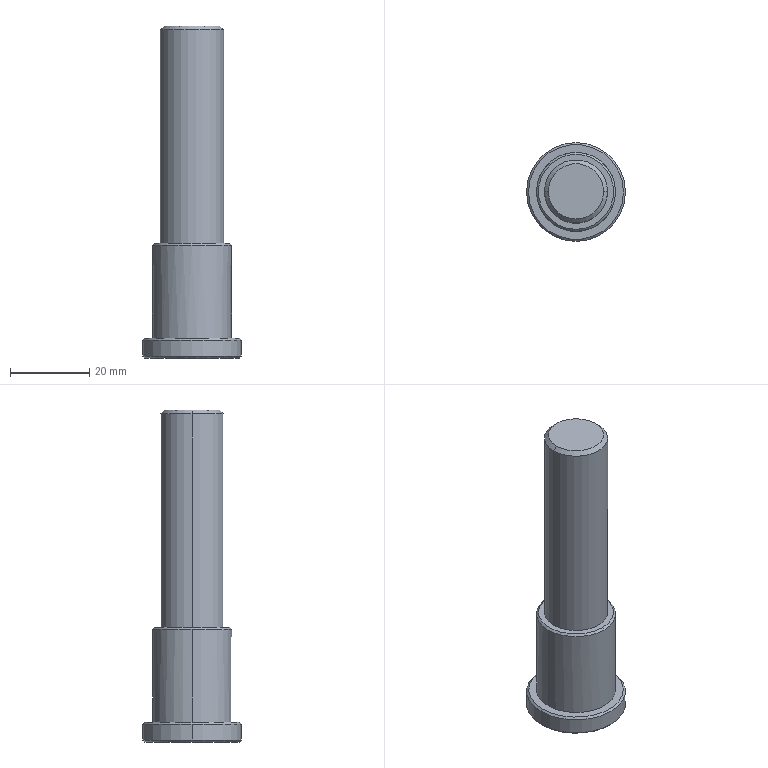Part | STEP file | 1 solid | 18 faces | box 25 x 25 x 84 mm | volume 21001 mm3 | cone 8 | cylinder 6 | plane 4 | commonest cylinder face diameters 16 x2 20 x2 25 x2
STEP:
#1=CARTESIAN_POINT('',(0.,0.,0.));
#2=DIRECTION('',(0.,0.,1.));
#3=DIRECTION('',(1.,0.,0.));
#4=AXIS2_PLACEMENT_3D('',#1,#2,#3);
#5=CARTESIAN_POINT('',(12.,0.,0.));
#6=VERTEX_POINT('',#5);
#7=CARTESIAN_POINT('',(-12.,0.,0.));
#8=VERTEX_POINT('',#7);
#9=CARTESIAN_POINT('',(0.,0.,0.));
#10=DIRECTION('',(0.,0.,1.));
#11=DIRECTION('',(1.,0.,0.));
#12=AXIS2_PLACEMENT_3D('',#9,#10,#11);
#13=CIRCLE('',#12,12.);
#14=CARTESIAN_POINT('',(0.,0.,0.));
#15=DIRECTION('',(0.,0.,1.));
#16=DIRECTION('',(1.,0.,0.));
#17=AXIS2_PLACEMENT_3D('',#14,#15,#16);
#18=PLANE('',#17);
#19=CARTESIAN_POINT('',(0.,0.));
#20=DIRECTION('',(1.,0.));
#21=AXIS2_PLACEMENT_2D('',#19,#20);
#22=CIRCLE('',#21,12.);
#23=(GEOMETRIC_REPRESENTATION_CONTEXT(2)PARAMETRIC_REPRESENTATION_CONTEXT()REPRESENTATION_CONTEXT('',''));
#24=DEFINITIONAL_REPRESENTATION('',(#22),#23);
#25=PCURVE('',#18,#24);
#26=CARTESIAN_POINT('',(0.,0.,0.5));
#27=DIRECTION('',(0.,0.,1.));
#28=DIRECTION('',(1.,0.,0.));
#29=AXIS2_PLACEMENT_3D('',#26,#27,#28);
#30=CONICAL_SURFACE('',#29,12.5,0.7854);
#31=CARTESIAN_POINT('',(0.,-0.5));
#32=DIRECTION('',(1.,0.));
#33=VECTOR('',#32,1.);
#34=LINE('',#31,#33);
#35=(GEOMETRIC_REPRESENTATION_CONTEXT(2)PARAMETRIC_REPRESENTATION_CONTEXT()REPRESENTATION_CONTEXT('',''));
#36=DEFINITIONAL_REPRESENTATION('',(#34),#35);
#37=PCURVE('',#30,#36);
#38=SURFACE_CURVE('',#13,(#25,#37),.PCURVE_S1.);
#39=EDGE_CURVE('',#6,#8,#38,.T.);
#40=ORIENTED_EDGE('',*,*,#39,.F.);
#41=CARTESIAN_POINT('',(0.,0.,0.));
#42=DIRECTION('',(0.,0.,1.));
#43=DIRECTION('',(1.,0.,0.));
#44=AXIS2_PLACEMENT_3D('',#41,#42,#43);
#45=CIRCLE('',#44,12.);
#46=CARTESIAN_POINT('',(0.,0.));
#47=DIRECTION('',(1.,0.));
#48=AXIS2_PLACEMENT_2D('',#46,#47);
#49=CIRCLE('',#48,12.);
#50=(GEOMETRIC_REPRESENTATION_CONTEXT(2)PARAMETRIC_REPRESENTATION_CONTEXT()REPRESENTATION_CONTEXT('',''));
#51=DEFINITIONAL_REPRESENTATION('',(#49),#50);
#52=PCURVE('',#18,#51);
#53=CARTESIAN_POINT('',(0.,0.,0.5));
#54=DIRECTION('',(0.,0.,1.));
#55=DIRECTION('',(1.,0.,0.));
#56=AXIS2_PLACEMENT_3D('',#53,#54,#55);
#57=CONICAL_SURFACE('',#56,12.5,0.7854);
#58=CARTESIAN_POINT('',(0.,-0.5));
#59=DIRECTION('',(1.,0.));
#60=VECTOR('',#59,1.);
#61=LINE('',#58,#60);
#62=(GEOMETRIC_REPRESENTATION_CONTEXT(2)PARAMETRIC_REPRESENTATION_CONTEXT()REPRESENTATION_CONTEXT('',''));
#63=DEFINITIONAL_REPRESENTATION('',(#61),#62);
#64=PCURVE('',#57,#63);
#65=SURFACE_CURVE('',#45,(#52,#64),.PCURVE_S1.);
#66=EDGE_CURVE('',#8,#6,#65,.T.);
#67=ORIENTED_EDGE('',*,*,#66,.F.);
#68=EDGE_LOOP('',(#40,#67));
#69=FACE_BOUND('',#68,.T.);
#70=ADVANCED_FACE('',(#69),#18,.F.);
#71=CARTESIAN_POINT('',(-12.5,0.,0.5));
#72=VERTEX_POINT('',#71);
#73=CARTESIAN_POINT('',(-12.5,0.,0.5));
#74=DIRECTION('',(-0.7071,0.,0.7071));
#75=VECTOR('',#74,1.);
#76=LINE('',#73,#75);
#77=CARTESIAN_POINT('',(3.142,0.));
#78=DIRECTION('',(0.,1.));
#79=VECTOR('',#78,1.);
#80=LINE('',#77,#79);
#81=(GEOMETRIC_REPRESENTATION_CONTEXT(2)PARAMETRIC_REPRESENTATION_CONTEXT()REPRESENTATION_CONTEXT('',''));
#82=DEFINITIONAL_REPRESENTATION('',(#80),#81);
#83=PCURVE('',#57,#82);
#84=CARTESIAN_POINT('',(3.142,0.));
#85=DIRECTION('',(0.,1.));
#86=VECTOR('',#85,1.);
#87=LINE('',#84,#86);
#88=(GEOMETRIC_REPRESENTATION_CONTEXT(2)PARAMETRIC_REPRESENTATION_CONTEXT()REPRESENTATION_CONTEXT('',''));
#89=DEFINITIONAL_REPRESENTATION('',(#87),#88);
#90=PCURVE('',#30,#89);
#91=SURFACE_CURVE('',#76,(#83,#90),.PCURVE_S1.);
#92=EDGE_CURVE('',#8,#72,#91,.T.);
#93=ORIENTED_EDGE('',*,*,#92,.F.);
#94=ORIENTED_EDGE('',*,*,#66,.T.);
#95=CARTESIAN_POINT('',(12.5,0.,0.5));
#96=VERTEX_POINT('',#95);
#97=CARTESIAN_POINT('',(12.5,0.,0.5));
#98=DIRECTION('',(0.7071,0.,0.7071));
#99=VECTOR('',#98,1.);
#100=LINE('',#97,#99);
#101=CARTESIAN_POINT('',(6.283,0.));
#102=DIRECTION('',(0.,1.));
#103=VECTOR('',#102,1.);
#104=LINE('',#101,#103);
#105=(GEOMETRIC_REPRESENTATION_CONTEXT(2)PARAMETRIC_REPRESENTATION_CONTEXT()REPRESENTATION_CONTEXT('',''));
#106=DEFINITIONAL_REPRESENTATION('',(#104),#105);
#107=PCURVE('',#57,#106);
#108=CARTESIAN_POINT('',(0.,0.));
#109=DIRECTION('',(0.,1.));
#110=VECTOR('',#109,1.);
#111=LINE('',#108,#110);
#112=(GEOMETRIC_REPRESENTATION_CONTEXT(2)PARAMETRIC_REPRESENTATION_CONTEXT()REPRESENTATION_CONTEXT('',''));
#113=DEFINITIONAL_REPRESENTATION('',(#111),#112);
#114=PCURVE('',#30,#113);
#115=SURFACE_CURVE('',#100,(#107,#114),.PCURVE_S1.);
#116=EDGE_CURVE('',#6,#96,#115,.T.);
#117=ORIENTED_EDGE('',*,*,#116,.T.);
#118=CARTESIAN_POINT('',(0.,0.,0.5));
#119=DIRECTION('',(0.,0.,1.));
#120=DIRECTION('',(-1.,0.,0.));
#121=AXIS2_PLACEMENT_3D('',#118,#119,#120);
#122=CIRCLE('',#121,12.5);
#123=CARTESIAN_POINT('',(3.142,0.));
#124=DIRECTION('',(1.,0.));
#125=VECTOR('',#124,1.);
#126=LINE('',#123,#125);
#127=(GEOMETRIC_REPRESENTATION_CONTEXT(2)PARAMETRIC_REPRESENTATION_CONTEXT()REPRESENTATION_CONTEXT('',''));
#128=DEFINITIONAL_REPRESENTATION('',(#126),#127);
#129=PCURVE('',#57,#128);
#130=CARTESIAN_POINT('',(0.,0.,5.));
#131=DIRECTION('',(0.,0.,-1.));
#132=DIRECTION('',(-1.,0.,0.));
#133=AXIS2_PLACEMENT_3D('',#130,#131,#132);
#134=CYLINDRICAL_SURFACE('',#133,12.5);
#135=CARTESIAN_POINT('',(6.283,4.5));
#136=DIRECTION('',(-1.,0.));
#137=VECTOR('',#136,1.);
#138=LINE('',#135,#137);
#139=(GEOMETRIC_REPRESENTATION_CONTEXT(2)PARAMETRIC_REPRESENTATION_CONTEXT()REPRESENTATION_CONTEXT('',''));
#140=DEFINITIONAL_REPRESENTATION('',(#138),#139);
#141=PCURVE('',#134,#140);
#142=SURFACE_CURVE('',#122,(#129,#141),.PCURVE_S1.);
#143=EDGE_CURVE('',#72,#96,#142,.T.);
#144=ORIENTED_EDGE('',*,*,#143,.F.);
#145=EDGE_LOOP('',(#93,#94,#117,#144));
#146=FACE_BOUND('',#145,.T.);
#147=ADVANCED_FACE('',(#146),#57,.T.);
#148=CARTESIAN_POINT('',(12.5,0.,4.5));
#149=VERTEX_POINT('',#148);
#150=CARTESIAN_POINT('',(12.5,0.,5.));
#151=DIRECTION('',(0.,0.,-1.));
#152=VECTOR('',#151,1.);
#153=LINE('',#150,#152);
#154=CARTESIAN_POINT('',(3.142,0.));
#155=DIRECTION('',(0.,1.));
#156=VECTOR('',#155,1.);
#157=LINE('',#154,#156);
#158=(GEOMETRIC_REPRESENTATION_CONTEXT(2)PARAMETRIC_REPRESENTATION_CONTEXT()REPRESENTATION_CONTEXT('',''));
#159=DEFINITIONAL_REPRESENTATION('',(#157),#158);
#160=PCURVE('',#134,#159);
#161=CARTESIAN_POINT('',(0.,0.,5.));
#162=DIRECTION('',(0.,0.,-1.));
#163=DIRECTION('',(-1.,0.,0.));
#164=AXIS2_PLACEMENT_3D('',#161,#162,#163);
#165=CYLINDRICAL_SURFACE('',#164,12.5);
#166=CARTESIAN_POINT('',(3.142,0.));
#167=DIRECTION('',(0.,1.));
#168=VECTOR('',#167,1.);
#169=LINE('',#166,#168);
#170=(GEOMETRIC_REPRESENTATION_CONTEXT(2)PARAMETRIC_REPRESENTATION_CONTEXT()REPRESENTATION_CONTEXT('',''));
#171=DEFINITIONAL_REPRESENTATION('',(#169),#170);
#172=PCURVE('',#165,#171);
#173=SURFACE_CURVE('',#153,(#160,#172),.PCURVE_S1.);
#174=EDGE_CURVE('',#149,#96,#173,.T.);
#175=ORIENTED_EDGE('',*,*,#174,.F.);
#176=CARTESIAN_POINT('',(-12.5,0.,4.5));
#177=VERTEX_POINT('',#176);
#178=CARTESIAN_POINT('',(0.,0.,4.5));
#179=DIRECTION('',(0.,0.,1.));
#180=DIRECTION('',(-1.,0.,0.));
#181=AXIS2_PLACEMENT_3D('',#178,#179,#180);
#182=CIRCLE('',#181,12.5);
#183=CARTESIAN_POINT('',(6.283,0.5));
#184=DIRECTION('',(-1.,0.));
#185=VECTOR('',#184,1.);
#186=LINE('',#183,#185);
#187=(GEOMETRIC_REPRESENTATION_CONTEXT(2)PARAMETRIC_REPRESENTATION_CONTEXT()REPRESENTATION_CONTEXT('',''));
#188=DEFINITIONAL_REPRESENTATION('',(#186),#187);
#189=PCURVE('',#134,#188);
#190=CARTESIAN_POINT('',(0.,0.,4.5));
#191=DIRECTION('',(0.,0.,-1.));
#192=DIRECTION('',(-1.,0.,0.));
#193=AXIS2_PLACEMENT_3D('',#190,#191,#192);
#194=CONICAL_SURFACE('',#193,12.5,0.7854);
#195=CARTESIAN_POINT('',(6.283,0.));
#196=DIRECTION('',(-1.,0.));
#197=VECTOR('',#196,1.);
#198=LINE('',#195,#197);
#199=(GEOMETRIC_REPRESENTATION_CONTEXT(2)PARAMETRIC_REPRESENTATION_CONTEXT()REPRESENTATION_CONTEXT('',''));
#200=DEFINITIONAL_REPRESENTATION('',(#198),#199);
#201=PCURVE('',#194,#200);
#202=SURFACE_CURVE('',#182,(#189,#201),.PCURVE_S1.);
#203=EDGE_CURVE('',#177,#149,#202,.T.);
#204=ORIENTED_EDGE('',*,*,#203,.F.);
#205=CARTESIAN_POINT('',(-12.5,0.,5.));
#206=DIRECTION('',(0.,0.,-1.));
#207=VECTOR('',#206,1.);
#208=LINE('',#205,#207);
#209=CARTESIAN_POINT('',(6.283,0.));
#210=DIRECTION('',(0.,1.));
#211=VECTOR('',#210,1.);
#212=LINE('',#209,#211);
#213=(GEOMETRIC_REPRESENTATION_CONTEXT(2)PARAMETRIC_REPRESENTATION_CONTEXT()REPRESENTATION_CONTEXT('',''));
#214=DEFINITIONAL_REPRESENTATION('',(#212),#213);
#215=PCURVE('',#134,#214);
#216=CARTESIAN_POINT('',(0.,0.));
#217=DIRECTION('',(0.,1.));
#218=VECTOR('',#217,1.);
#219=LINE('',#216,#218);
#220=(GEOMETRIC_REPRESENTATION_CONTEXT(2)PARAMETRIC_REPRESENTATION_CONTEXT()REPRESENTATION_CONTEXT('',''));
#221=DEFINITIONAL_REPRESENTATION('',(#219),#220);
#222=PCURVE('',#165,#221);
#223=SURFACE_CURVE('',#208,(#215,#222),.PCURVE_S1.);
#224=EDGE_CURVE('',#177,#72,#223,.T.);
#225=ORIENTED_EDGE('',*,*,#224,.T.);
#226=ORIENTED_EDGE('',*,*,#143,.T.);
#227=EDGE_LOOP('',(#175,#204,#225,#226));
#228=FACE_BOUND('',#227,.T.);
#229=ADVANCED_FACE('',(#228),#134,.T.);
#230=CARTESIAN_POINT('',(12.,0.,5.));
#231=VERTEX_POINT('',#230);
#232=CARTESIAN_POINT('',(12.5,0.,4.5));
#233=DIRECTION('',(0.7071,0.,-0.7071));
#234=VECTOR('',#233,1.);
#235=LINE('',#232,#234);
#236=CARTESIAN_POINT('',(3.142,0.));
#237=DIRECTION('',(0.,1.));
#238=VECTOR('',#237,1.);
#239=LINE('',#236,#238);
#240=(GEOMETRIC_REPRESENTATION_CONTEXT(2)PARAMETRIC_REPRESENTATION_CONTEXT()REPRESENTATION_CONTEXT('',''));
#241=DEFINITIONAL_REPRESENTATION('',(#239),#240);
#242=PCURVE('',#194,#241);
#243=CARTESIAN_POINT('',(0.,0.,4.5));
#244=DIRECTION('',(0.,0.,-1.));
#245=DIRECTION('',(-1.,0.,0.));
#246=AXIS2_PLACEMENT_3D('',#243,#244,#245);
#247=CONICAL_SURFACE('',#246,12.5,0.7854);
#248=CARTESIAN_POINT('',(3.142,0.));
#249=DIRECTION('',(0.,1.));
#250=VECTOR('',#249,1.);
#251=LINE('',#248,#250);
#252=(GEOMETRIC_REPRESENTATION_CONTEXT(2)PARAMETRIC_REPRESENTATION_CONTEXT()REPRESENTATION_CONTEXT('',''));
#253=DEFINITIONAL_REPRESENTATION('',(#251),#252);
#254=PCURVE('',#247,#253);
#255=SURFACE_CURVE('',#235,(#242,#254),.PCURVE_S1.);
#256=EDGE_CURVE('',#231,#149,#255,.T.);
#257=ORIENTED_EDGE('',*,*,#256,.F.);
#258=CARTESIAN_POINT('',(-12.,0.,5.));
#259=VERTEX_POINT('',#258);
#260=CARTESIAN_POINT('',(0.,0.,5.));
#261=DIRECTION('',(0.,0.,1.));
#262=DIRECTION('',(-1.,0.,0.));
#263=AXIS2_PLACEMENT_3D('',#260,#261,#262);
#264=CIRCLE('',#263,12.);
#265=CARTESIAN_POINT('',(6.283,-0.5));
#266=DIRECTION('',(-1.,0.));
#267=VECTOR('',#266,1.);
#268=LINE('',#265,#267);
#269=(GEOMETRIC_REPRESENTATION_CONTEXT(2)PARAMETRIC_REPRESENTATION_CONTEXT()REPRESENTATION_CONTEXT('',''));
#270=DEFINITIONAL_REPRESENTATION('',(#268),#269);
#271=PCURVE('',#194,#270);
#272=CARTESIAN_POINT('',(0.,0.,5.));
#273=DIRECTION('',(0.,0.,1.));
#274=DIRECTION('',(1.,0.,0.));
#275=AXIS2_PLACEMENT_3D('',#272,#273,#274);
#276=PLANE('',#275);
#277=CARTESIAN_POINT('',(0.,0.));
#278=DIRECTION('',(-1.,0.));
#279=AXIS2_PLACEMENT_2D('',#277,#278);
#280=CIRCLE('',#279,12.);
#281=(GEOMETRIC_REPRESENTATION_CONTEXT(2)PARAMETRIC_REPRESENTATION_CONTEXT()REPRESENTATION_CONTEXT('',''));
#282=DEFINITIONAL_REPRESENTATION('',(#280),#281);
#283=PCURVE('',#276,#282);
#284=SURFACE_CURVE('',#264,(#271,#283),.PCURVE_S1.);
#285=EDGE_CURVE('',#259,#231,#284,.T.);
#286=ORIENTED_EDGE('',*,*,#285,.F.);
#287=CARTESIAN_POINT('',(-12.5,0.,4.5));
#288=DIRECTION('',(-0.7071,0.,-0.7071));
#289=VECTOR('',#288,1.);
#290=LINE('',#287,#289);
#291=CARTESIAN_POINT('',(6.283,0.));
#292=DIRECTION('',(0.,1.));
#293=VECTOR('',#292,1.);
#294=LINE('',#291,#293);
#295=(GEOMETRIC_REPRESENTATION_CONTEXT(2)PARAMETRIC_REPRESENTATION_CONTEXT()REPRESENTATION_CONTEXT('',''));
#296=DEFINITIONAL_REPRESENTATION('',(#294),#295);
#297=PCURVE('',#194,#296);
#298=CARTESIAN_POINT('',(0.,0.));
#299=DIRECTION('',(0.,1.));
#300=VECTOR('',#299,1.);
#301=LINE('',#298,#300);
#302=(GEOMETRIC_REPRESENTATION_CONTEXT(2)PARAMETRIC_REPRESENTATION_CONTEXT()REPRESENTATION_CONTEXT('',''));
#303=DEFINITIONAL_REPRESENTATION('',(#301),#302);
#304=PCURVE('',#247,#303);
#305=SURFACE_CURVE('',#290,(#297,#304),.PCURVE_S1.);
#306=EDGE_CURVE('',#259,#177,#305,.T.);
#307=ORIENTED_EDGE('',*,*,#306,.T.);
#308=ORIENTED_EDGE('',*,*,#203,.T.);
#309=EDGE_LOOP('',(#257,#286,#307,#308));
#310=FACE_BOUND('',#309,.T.);
#311=ADVANCED_FACE('',(#310),#194,.T.);
#312=CARTESIAN_POINT('',(-10.,0.,5.));
#313=VERTEX_POINT('',#312);
#314=CARTESIAN_POINT('',(10.,0.,5.));
#315=VERTEX_POINT('',#314);
#316=CARTESIAN_POINT('',(0.,0.,5.));
#317=DIRECTION('',(0.,0.,1.));
#318=DIRECTION('',(-1.,0.,0.));
#319=AXIS2_PLACEMENT_3D('',#316,#317,#318);
#320=CIRCLE('',#319,10.);
#321=CARTESIAN_POINT('',(0.,0.));
#322=DIRECTION('',(-1.,0.));
#323=AXIS2_PLACEMENT_2D('',#321,#322);
#324=CIRCLE('',#323,10.);
#325=(GEOMETRIC_REPRESENTATION_CONTEXT(2)PARAMETRIC_REPRESENTATION_CONTEXT()REPRESENTATION_CONTEXT('',''));
#326=DEFINITIONAL_REPRESENTATION('',(#324),#325);
#327=PCURVE('',#276,#326);
#328=CARTESIAN_POINT('',(0.,0.,29.));
#329=DIRECTION('',(0.,0.,-1.));
#330=DIRECTION('',(-1.,0.,0.));
#331=AXIS2_PLACEMENT_3D('',#328,#329,#330);
#332=CYLINDRICAL_SURFACE('',#331,10.);
#333=CARTESIAN_POINT('',(6.283,24.));
#334=DIRECTION('',(-1.,0.));
#335=VECTOR('',#334,1.);
#336=LINE('',#333,#335);
#337=(GEOMETRIC_REPRESENTATION_CONTEXT(2)PARAMETRIC_REPRESENTATION_CONTEXT()REPRESENTATION_CONTEXT('',''));
#338=DEFINITIONAL_REPRESENTATION('',(#336),#337);
#339=PCURVE('',#332,#338);
#340=SURFACE_CURVE('',#320,(#327,#339),.PCURVE_S1.);
#341=EDGE_CURVE('',#313,#315,#340,.T.);
#342=ORIENTED_EDGE('',*,*,#341,.F.);
#343=CARTESIAN_POINT('',(0.,0.,5.));
#344=DIRECTION('',(0.,0.,1.));
#345=DIRECTION('',(-1.,0.,0.));
#346=AXIS2_PLACEMENT_3D('',#343,#344,#345);
#347=CIRCLE('',#346,10.);
#348=CARTESIAN_POINT('',(0.,0.));
#349=DIRECTION('',(-1.,0.));
#350=AXIS2_PLACEMENT_2D('',#348,#349);
#351=CIRCLE('',#350,10.);
#352=(GEOMETRIC_REPRESENTATION_CONTEXT(2)PARAMETRIC_REPRESENTATION_CONTEXT()REPRESENTATION_CONTEXT('',''));
#353=DEFINITIONAL_REPRESENTATION('',(#351),#352);
#354=PCURVE('',#276,#353);
#355=CARTESIAN_POINT('',(0.,0.,29.));
#356=DIRECTION('',(0.,0.,-1.));
#357=DIRECTION('',(-1.,0.,0.));
#358=AXIS2_PLACEMENT_3D('',#355,#356,#357);
#359=CYLINDRICAL_SURFACE('',#358,10.);
#360=CARTESIAN_POINT('',(6.283,24.));
#361=DIRECTION('',(-1.,0.));
#362=VECTOR('',#361,1.);
#363=LINE('',#360,#362);
#364=(GEOMETRIC_REPRESENTATION_CONTEXT(2)PARAMETRIC_REPRESENTATION_CONTEXT()REPRESENTATION_CONTEXT('',''));
#365=DEFINITIONAL_REPRESENTATION('',(#363),#364);
#366=PCURVE('',#359,#365);
#367=SURFACE_CURVE('',#347,(#354,#366),.PCURVE_S1.);
#368=EDGE_CURVE('',#315,#313,#367,.T.);
#369=ORIENTED_EDGE('',*,*,#368,.F.);
#370=EDGE_LOOP('',(#342,#369));
#371=FACE_BOUND('',#370,.T.);
#372=ORIENTED_EDGE('',*,*,#285,.T.);
#373=CARTESIAN_POINT('',(0.,0.,5.));
#374=DIRECTION('',(0.,0.,1.));
#375=DIRECTION('',(-1.,0.,0.));
#376=AXIS2_PLACEMENT_3D('',#373,#374,#375);
#377=CIRCLE('',#376,12.);
#378=CARTESIAN_POINT('',(0.,0.));
#379=DIRECTION('',(-1.,0.));
#380=AXIS2_PLACEMENT_2D('',#378,#379);
#381=CIRCLE('',#380,12.);
#382=(GEOMETRIC_REPRESENTATION_CONTEXT(2)PARAMETRIC_REPRESENTATION_CONTEXT()REPRESENTATION_CONTEXT('',''));
#383=DEFINITIONAL_REPRESENTATION('',(#381),#382);
#384=PCURVE('',#276,#383);
#385=CARTESIAN_POINT('',(6.283,-0.5));
#386=DIRECTION('',(-1.,0.));
#387=VECTOR('',#386,1.);
#388=LINE('',#385,#387);
#389=(GEOMETRIC_REPRESENTATION_CONTEXT(2)PARAMETRIC_REPRESENTATION_CONTEXT()REPRESENTATION_CONTEXT('',''));
#390=DEFINITIONAL_REPRESENTATION('',(#388),#389);
#391=PCURVE('',#247,#390);
#392=SURFACE_CURVE('',#377,(#384,#391),.PCURVE_S1.);
#393=EDGE_CURVE('',#231,#259,#392,.T.);
#394=ORIENTED_EDGE('',*,*,#393,.T.);
#395=EDGE_LOOP('',(#372,#394));
#396=FACE_BOUND('',#395,.T.);
#397=ADVANCED_FACE('',(#371,#396),#276,.T.);
#398=CARTESIAN_POINT('',(10.,0.,28.5));
#399=VERTEX_POINT('',#398);
#400=CARTESIAN_POINT('',(10.,0.,29.));
#401=DIRECTION('',(0.,0.,-1.));
#402=VECTOR('',#401,1.);
#403=LINE('',#400,#402);
#404=CARTESIAN_POINT('',(3.142,0.));
#405=DIRECTION('',(0.,1.));
#406=VECTOR('',#405,1.);
#407=LINE('',#404,#406);
#408=(GEOMETRIC_REPRESENTATION_CONTEXT(2)PARAMETRIC_REPRESENTATION_CONTEXT()REPRESENTATION_CONTEXT('',''));
#409=DEFINITIONAL_REPRESENTATION('',(#407),#408);
#410=PCURVE('',#332,#409);
#411=CARTESIAN_POINT('',(3.142,0.));
#412=DIRECTION('',(0.,1.));
#413=VECTOR('',#412,1.);
#414=LINE('',#411,#413);
#415=(GEOMETRIC_REPRESENTATION_CONTEXT(2)PARAMETRIC_REPRESENTATION_CONTEXT()REPRESENTATION_CONTEXT('',''));
#416=DEFINITIONAL_REPRESENTATION('',(#414),#415);
#417=PCURVE('',#359,#416);
#418=SURFACE_CURVE('',#403,(#410,#417),.PCURVE_S1.);
#419=EDGE_CURVE('',#399,#315,#418,.T.);
#420=ORIENTED_EDGE('',*,*,#419,.F.);
#421=CARTESIAN_POINT('',(0.,-10.,28.5));
#422=VERTEX_POINT('',#421);
#423=CARTESIAN_POINT('',(0.,0.,28.5));
#424=DIRECTION('',(0.,0.,1.));
#425=DIRECTION('',(-1.,0.,0.));
#426=AXIS2_PLACEMENT_3D('',#423,#424,#425);
#427=CIRCLE('',#426,10.);
#428=CARTESIAN_POINT('',(6.283,0.5));
#429=DIRECTION('',(-1.,0.));
#430=VECTOR('',#429,1.);
#431=LINE('',#428,#430);
#432=(GEOMETRIC_REPRESENTATION_CONTEXT(2)PARAMETRIC_REPRESENTATION_CONTEXT()REPRESENTATION_CONTEXT('',''));
#433=DEFINITIONAL_REPRESENTATION('',(#431),#432);
#434=PCURVE('',#332,#433);
#435=CARTESIAN_POINT('',(0.,0.,28.5));
#436=DIRECTION('',(0.,0.,-1.));
#437=DIRECTION('',(0.,1.,0.));
#438=AXIS2_PLACEMENT_3D('',#435,#436,#437);
#439=CONICAL_SURFACE('',#438,10.,0.7854);
#440=CARTESIAN_POINT('',(4.712,0.));
#441=DIRECTION('',(-1.,0.));
#442=VECTOR('',#441,1.);
#443=LINE('',#440,#442);
#444=(GEOMETRIC_REPRESENTATION_CONTEXT(2)PARAMETRIC_REPRESENTATION_CONTEXT()REPRESENTATION_CONTEXT('',''));
#445=DEFINITIONAL_REPRESENTATION('',(#443),#444);
#446=PCURVE('',#439,#445);
#447=SURFACE_CURVE('',#427,(#434,#446),.PCURVE_S1.);
#448=EDGE_CURVE('',#422,#399,#447,.T.);
#449=ORIENTED_EDGE('',*,*,#448,.F.);
#450=CARTESIAN_POINT('',(-10.,0.,28.5));
#451=VERTEX_POINT('',#450);
#452=CARTESIAN_POINT('',(0.,0.,28.5));
#453=DIRECTION('',(0.,0.,1.));
#454=DIRECTION('',(-1.,0.,0.));
#455=AXIS2_PLACEMENT_3D('',#452,#453,#454);
#456=CIRCLE('',#455,10.);
#457=CARTESIAN_POINT('',(6.283,0.5));
#458=DIRECTION('',(-1.,0.));
#459=VECTOR('',#458,1.);
#460=LINE('',#457,#459);
#461=(GEOMETRIC_REPRESENTATION_CONTEXT(2)PARAMETRIC_REPRESENTATION_CONTEXT()REPRESENTATION_CONTEXT('',''));
#462=DEFINITIONAL_REPRESENTATION('',(#460),#461);
#463=PCURVE('',#332,#462);
#464=CARTESIAN_POINT('',(0.,0.,28.5));
#465=DIRECTION('',(0.,0.,-1.));
#466=DIRECTION('',(0.,1.,0.));
#467=AXIS2_PLACEMENT_3D('',#464,#465,#466);
#468=CONICAL_SURFACE('',#467,10.,0.7854);
#469=CARTESIAN_POINT('',(4.712,0.));
#470=DIRECTION('',(-1.,0.));
#471=VECTOR('',#470,1.);
#472=LINE('',#469,#471);
#473=(GEOMETRIC_REPRESENTATION_CONTEXT(2)PARAMETRIC_REPRESENTATION_CONTEXT()REPRESENTATION_CONTEXT('',''));
#474=DEFINITIONAL_REPRESENTATION('',(#472),#473);
#475=PCURVE('',#468,#474);
#476=SURFACE_CURVE('',#456,(#463,#475),.PCURVE_S1.);
#477=EDGE_CURVE('',#451,#422,#476,.T.);
#478=ORIENTED_EDGE('',*,*,#477,.F.);
#479=CARTESIAN_POINT('',(-10.,0.,29.));
#480=DIRECTION('',(0.,0.,-1.));
#481=VECTOR('',#480,1.);
#482=LINE('',#479,#481);
#483=CARTESIAN_POINT('',(6.283,0.));
#484=DIRECTION('',(0.,1.));
#485=VECTOR('',#484,1.);
#486=LINE('',#483,#485);
#487=(GEOMETRIC_REPRESENTATION_CONTEXT(2)PARAMETRIC_REPRESENTATION_CONTEXT()REPRESENTATION_CONTEXT('',''));
#488=DEFINITIONAL_REPRESENTATION('',(#486),#487);
#489=PCURVE('',#332,#488);
#490=CARTESIAN_POINT('',(0.,0.));
#491=DIRECTION('',(0.,1.));
#492=VECTOR('',#491,1.);
#493=LINE('',#490,#492);
#494=(GEOMETRIC_REPRESENTATION_CONTEXT(2)PARAMETRIC_REPRESENTATION_CONTEXT()REPRESENTATION_CONTEXT('',''));
#495=DEFINITIONAL_REPRESENTATION('',(#493),#494);
#496=PCURVE('',#359,#495);
#497=SURFACE_CURVE('',#482,(#489,#496),.PCURVE_S1.);
#498=EDGE_CURVE('',#451,#313,#497,.T.);
#499=ORIENTED_EDGE('',*,*,#498,.T.);
#500=ORIENTED_EDGE('',*,*,#341,.T.);
#501=EDGE_LOOP('',(#420,#449,#478,#499,#500));
#502=FACE_BOUND('',#501,.T.);
#503=ADVANCED_FACE('',(#502),#332,.T.);
#504=CARTESIAN_POINT('',(-7.,0.,84.));
#505=VERTEX_POINT('',#504);
#506=CARTESIAN_POINT('',(7.,0.,84.));
#507=VERTEX_POINT('',#506);
#508=CARTESIAN_POINT('',(0.,0.,84.));
#509=DIRECTION('',(0.,0.,-1.));
#510=DIRECTION('',(-1.,0.,0.));
#511=AXIS2_PLACEMENT_3D('',#508,#509,#510);
#512=CIRCLE('',#511,7.);
#513=CARTESIAN_POINT('',(0.,0.,84.));
#514=DIRECTION('',(0.,0.,1.));
#515=DIRECTION('',(1.,0.,0.));
#516=AXIS2_PLACEMENT_3D('',#513,#514,#515);
#517=PLANE('',#516);
#518=CARTESIAN_POINT('',(-7.,0.));
#519=CARTESIAN_POINT('',(-7.,12.124));
#520=CARTESIAN_POINT('',(3.5,6.062));
#521=CARTESIAN_POINT('',(14.,0.));
#522=CARTESIAN_POINT('',(3.5,-6.062));
#523=CARTESIAN_POINT('',(-7.,-12.124));
#524=CARTESIAN_POINT('',(-7.,0.));
#525=(BOUNDED_CURVE()B_SPLINE_CURVE(2,(#518,#519,#520,#521,#522,#523,#524),.UNSPECIFIED.,.T.,.F.)B_SPLINE_CURVE_WITH_KNOTS((1,2,2,2,2,1),(-2.094,0.,2.094,4.189,6.283,8.378),.UNSPECIFIED.)CURVE()GEOMETRIC_REPRESENTATION_ITEM()RATIONAL_B_SPLINE_CURVE((1.,0.5,1.,0.5,1.,0.5,1.))REPRESENTATION_ITEM(''));
#526=(GEOMETRIC_REPRESENTATION_CONTEXT(2)PARAMETRIC_REPRESENTATION_CONTEXT()REPRESENTATION_CONTEXT('',''));
#527=DEFINITIONAL_REPRESENTATION('',(#525),#526);
#528=PCURVE('',#517,#527);
#529=CARTESIAN_POINT('',(0.,0.,83.));
#530=DIRECTION('',(0.,0.,-1.));
#531=DIRECTION('',(-1.,0.,0.));
#532=AXIS2_PLACEMENT_3D('',#529,#530,#531);
#533=CONICAL_SURFACE('',#532,8.,0.7854);
#534=CARTESIAN_POINT('',(0.,-1.));
#535=DIRECTION('',(1.,0.));
#536=VECTOR('',#535,1.);
#537=LINE('',#534,#536);
#538=(GEOMETRIC_REPRESENTATION_CONTEXT(2)PARAMETRIC_REPRESENTATION_CONTEXT()REPRESENTATION_CONTEXT('',''));
#539=DEFINITIONAL_REPRESENTATION('',(#537),#538);
#540=PCURVE('',#533,#539);
#541=SURFACE_CURVE('',#512,(#528,#540),.PCURVE_S1.);
#542=EDGE_CURVE('',#505,#507,#541,.T.);
#543=ORIENTED_EDGE('',*,*,#542,.F.);
#544=CARTESIAN_POINT('',(0.,0.,84.));
#545=DIRECTION('',(0.,0.,-1.));
#546=DIRECTION('',(-1.,0.,0.));
#547=AXIS2_PLACEMENT_3D('',#544,#545,#546);
#548=CIRCLE('',#547,7.);
#549=CARTESIAN_POINT('',(-7.,0.));
#550=CARTESIAN_POINT('',(-7.,12.124));
#551=CARTESIAN_POINT('',(3.5,6.062));
#552=CARTESIAN_POINT('',(14.,0.));
#553=CARTESIAN_POINT('',(3.5,-6.062));
#554=CARTESIAN_POINT('',(-7.,-12.124));
#555=CARTESIAN_POINT('',(-7.,0.));
#556=(BOUNDED_CURVE()B_SPLINE_CURVE(2,(#549,#550,#551,#552,#553,#554,#555),.UNSPECIFIED.,.T.,.F.)B_SPLINE_CURVE_WITH_KNOTS((1,2,2,2,2,1),(-2.094,0.,2.094,4.189,6.283,8.378),.UNSPECIFIED.)CURVE()GEOMETRIC_REPRESENTATION_ITEM()RATIONAL_B_SPLINE_CURVE((1.,0.5,1.,0.5,1.,0.5,1.))REPRESENTATION_ITEM(''));
#557=(GEOMETRIC_REPRESENTATION_CONTEXT(2)PARAMETRIC_REPRESENTATION_CONTEXT()REPRESENTATION_CONTEXT('',''));
#558=DEFINITIONAL_REPRESENTATION('',(#556),#557);
#559=PCURVE('',#517,#558);
#560=CARTESIAN_POINT('',(0.,0.,83.));
#561=DIRECTION('',(0.,0.,-1.));
#562=DIRECTION('',(-1.,0.,0.));
#563=AXIS2_PLACEMENT_3D('',#560,#561,#562);
#564=CONICAL_SURFACE('',#563,8.,0.7854);
#565=CARTESIAN_POINT('',(0.,-1.));
#566=DIRECTION('',(1.,0.));
#567=VECTOR('',#566,1.);
#568=LINE('',#565,#567);
#569=(GEOMETRIC_REPRESENTATION_CONTEXT(2)PARAMETRIC_REPRESENTATION_CONTEXT()REPRESENTATION_CONTEXT('',''));
#570=DEFINITIONAL_REPRESENTATION('',(#568),#569);
#571=PCURVE('',#564,#570);
#572=SURFACE_CURVE('',#548,(#559,#571),.PCURVE_S1.);
#573=EDGE_CURVE('',#507,#505,#572,.T.);
#574=ORIENTED_EDGE('',*,*,#573,.F.);
#575=EDGE_LOOP('',(#543,#574));
#576=FACE_BOUND('',#575,.T.);
#577=ADVANCED_FACE('',(#576),#517,.T.);
#578=CARTESIAN_POINT('',(0.,-9.5,29.));
#579=VERTEX_POINT('',#578);
#580=CARTESIAN_POINT('',(0.,-10.,28.5));
#581=DIRECTION('',(0.,-0.7071,-0.7071));
#582=VECTOR('',#581,1.);
#583=LINE('',#580,#582);
#584=CARTESIAN_POINT('',(3.142,0.));
#585=DIRECTION('',(0.,1.));
#586=VECTOR('',#585,1.);
#587=LINE('',#584,#586);
#588=(GEOMETRIC_REPRESENTATION_CONTEXT(2)PARAMETRIC_REPRESENTATION_CONTEXT()REPRESENTATION_CONTEXT('',''));
#589=DEFINITIONAL_REPRESENTATION('',(#587),#588);
#590=PCURVE('',#468,#589);
#591=CARTESIAN_POINT('',(3.142,0.));
#592=DIRECTION('',(0.,1.));
#593=VECTOR('',#592,1.);
#594=LINE('',#591,#593);
#595=(GEOMETRIC_REPRESENTATION_CONTEXT(2)PARAMETRIC_REPRESENTATION_CONTEXT()REPRESENTATION_CONTEXT('',''));
#596=DEFINITIONAL_REPRESENTATION('',(#594),#595);
#597=PCURVE('',#439,#596);
#598=SURFACE_CURVE('',#583,(#590,#597),.PCURVE_S1.);
#599=EDGE_CURVE('',#579,#422,#598,.T.);
#600=ORIENTED_EDGE('',*,*,#599,.F.);
#601=CARTESIAN_POINT('',(0.,9.5,29.));
#602=VERTEX_POINT('',#601);
#603=CARTESIAN_POINT('',(0.,0.,29.));
#604=DIRECTION('',(0.,0.,1.));
#605=DIRECTION('',(0.,1.,0.));
#606=AXIS2_PLACEMENT_3D('',#603,#604,#605);
#607=CIRCLE('',#606,9.5);
#608=CARTESIAN_POINT('',(6.283,-0.5));
#609=DIRECTION('',(-1.,0.));
#610=VECTOR('',#609,1.);
#611=LINE('',#608,#610);
#612=(GEOMETRIC_REPRESENTATION_CONTEXT(2)PARAMETRIC_REPRESENTATION_CONTEXT()REPRESENTATION_CONTEXT('',''));
#613=DEFINITIONAL_REPRESENTATION('',(#611),#612);
#614=PCURVE('',#468,#613);
#615=CARTESIAN_POINT('',(0.,0.,29.));
#616=DIRECTION('',(0.,0.,1.));
#617=DIRECTION('',(1.,0.,0.));
#618=AXIS2_PLACEMENT_3D('',#615,#616,#617);
#619=PLANE('',#618);
#620=CARTESIAN_POINT('',(0.,0.));
#621=DIRECTION('',(0.,1.));
#622=AXIS2_PLACEMENT_2D('',#620,#621);
#623=CIRCLE('',#622,9.5);
#624=(GEOMETRIC_REPRESENTATION_CONTEXT(2)PARAMETRIC_REPRESENTATION_CONTEXT()REPRESENTATION_CONTEXT('',''));
#625=DEFINITIONAL_REPRESENTATION('',(#623),#624);
#626=PCURVE('',#619,#625);
#627=SURFACE_CURVE('',#607,(#614,#626),.PCURVE_S1.);
#628=EDGE_CURVE('',#602,#579,#627,.T.);
#629=ORIENTED_EDGE('',*,*,#628,.F.);
#630=CARTESIAN_POINT('',(0.,10.,28.5));
#631=VERTEX_POINT('',#630);
#632=CARTESIAN_POINT('',(0.,10.,28.5));
#633=DIRECTION('',(0.,0.7071,-0.7071));
#634=VECTOR('',#633,1.);
#635=LINE('',#632,#634);
#636=CARTESIAN_POINT('',(6.283,0.));
#637=DIRECTION('',(0.,1.));
#638=VECTOR('',#637,1.);
#639=LINE('',#636,#638);
#640=(GEOMETRIC_REPRESENTATION_CONTEXT(2)PARAMETRIC_REPRESENTATION_CONTEXT()REPRESENTATION_CONTEXT('',''));
#641=DEFINITIONAL_REPRESENTATION('',(#639),#640);
#642=PCURVE('',#468,#641);
#643=CARTESIAN_POINT('',(0.,0.));
#644=DIRECTION('',(0.,1.));
#645=VECTOR('',#644,1.);
#646=LINE('',#643,#645);
#647=(GEOMETRIC_REPRESENTATION_CONTEXT(2)PARAMETRIC_REPRESENTATION_CONTEXT()REPRESENTATION_CONTEXT('',''));
#648=DEFINITIONAL_REPRESENTATION('',(#646),#647);
#649=PCURVE('',#439,#648);
#650=SURFACE_CURVE('',#635,(#642,#649),.PCURVE_S1.);
#651=EDGE_CURVE('',#602,#631,#650,.T.);
#652=ORIENTED_EDGE('',*,*,#651,.T.);
#653=CARTESIAN_POINT('',(0.,0.,28.5));
#654=DIRECTION('',(0.,0.,1.));
#655=DIRECTION('',(-1.,0.,0.));
#656=AXIS2_PLACEMENT_3D('',#653,#654,#655);
#657=CIRCLE('',#656,10.);
#658=CARTESIAN_POINT('',(10.996,0.));
#659=DIRECTION('',(-1.,0.));
#660=VECTOR('',#659,1.);
#661=LINE('',#658,#660);
#662=(GEOMETRIC_REPRESENTATION_CONTEXT(2)PARAMETRIC_REPRESENTATION_CONTEXT()REPRESENTATION_CONTEXT('',''));
#663=DEFINITIONAL_REPRESENTATION('',(#661),#662);
#664=PCURVE('',#468,#663);
#665=CARTESIAN_POINT('',(6.283,0.5));
#666=DIRECTION('',(-1.,0.));
#667=VECTOR('',#666,1.);
#668=LINE('',#665,#667);
#669=(GEOMETRIC_REPRESENTATION_CONTEXT(2)PARAMETRIC_REPRESENTATION_CONTEXT()REPRESENTATION_CONTEXT('',''));
#670=DEFINITIONAL_REPRESENTATION('',(#668),#669);
#671=PCURVE('',#359,#670);
#672=SURFACE_CURVE('',#657,(#664,#671),.PCURVE_S1.);
#673=EDGE_CURVE('',#631,#451,#672,.T.);
#674=ORIENTED_EDGE('',*,*,#673,.T.);
#675=ORIENTED_EDGE('',*,*,#477,.T.);
#676=EDGE_LOOP('',(#600,#629,#652,#674,#675));
#677=FACE_BOUND('',#676,.T.);
#678=ADVANCED_FACE('',(#677),#468,.T.);
#679=CARTESIAN_POINT('',(8.,0.,83.));
#680=VERTEX_POINT('',#679);
#681=CARTESIAN_POINT('',(8.,0.,83.));
#682=DIRECTION('',(0.7071,0.,-0.7071));
#683=VECTOR('',#682,1.);
#684=LINE('',#681,#683);
#685=CARTESIAN_POINT('',(3.142,0.));
#686=DIRECTION('',(0.,1.));
#687=VECTOR('',#686,1.);
#688=LINE('',#685,#687);
#689=(GEOMETRIC_REPRESENTATION_CONTEXT(2)PARAMETRIC_REPRESENTATION_CONTEXT()REPRESENTATION_CONTEXT('',''));
#690=DEFINITIONAL_REPRESENTATION('',(#688),#689);
#691=PCURVE('',#564,#690);
#692=CARTESIAN_POINT('',(3.142,0.));
#693=DIRECTION('',(0.,1.));
#694=VECTOR('',#693,1.);
#695=LINE('',#692,#694);
#696=(GEOMETRIC_REPRESENTATION_CONTEXT(2)PARAMETRIC_REPRESENTATION_CONTEXT()REPRESENTATION_CONTEXT('',''));
#697=DEFINITIONAL_REPRESENTATION('',(#695),#696);
#698=PCURVE('',#533,#697);
#699=SURFACE_CURVE('',#684,(#691,#698),.PCURVE_S1.);
#700=EDGE_CURVE('',#507,#680,#699,.T.);
#701=ORIENTED_EDGE('',*,*,#700,.F.);
#702=ORIENTED_EDGE('',*,*,#573,.T.);
#703=CARTESIAN_POINT('',(-8.,0.,83.));
#704=VERTEX_POINT('',#703);
#705=CARTESIAN_POINT('',(-8.,0.,83.));
#706=DIRECTION('',(-0.7071,0.,-0.7071));
#707=VECTOR('',#706,1.);
#708=LINE('',#705,#707);
#709=CARTESIAN_POINT('',(6.283,0.));
#710=DIRECTION('',(0.,1.));
#711=VECTOR('',#710,1.);
#712=LINE('',#709,#711);
#713=(GEOMETRIC_REPRESENTATION_CONTEXT(2)PARAMETRIC_REPRESENTATION_CONTEXT()REPRESENTATION_CONTEXT('',''));
#714=DEFINITIONAL_REPRESENTATION('',(#712),#713);
#715=PCURVE('',#564,#714);
#716=CARTESIAN_POINT('',(0.,0.));
#717=DIRECTION('',(0.,1.));
#718=VECTOR('',#717,1.);
#719=LINE('',#716,#718);
#720=(GEOMETRIC_REPRESENTATION_CONTEXT(2)PARAMETRIC_REPRESENTATION_CONTEXT()REPRESENTATION_CONTEXT('',''));
#721=DEFINITIONAL_REPRESENTATION('',(#719),#720);
#722=PCURVE('',#533,#721);
#723=SURFACE_CURVE('',#708,(#715,#722),.PCURVE_S1.);
#724=EDGE_CURVE('',#505,#704,#723,.T.);
#725=ORIENTED_EDGE('',*,*,#724,.T.);
#726=CARTESIAN_POINT('',(0.,0.,83.));
#727=DIRECTION('',(0.,0.,-1.));
#728=DIRECTION('',(-1.,0.,0.));
#729=AXIS2_PLACEMENT_3D('',#726,#727,#728);
#730=CIRCLE('',#729,8.);
#731=CARTESIAN_POINT('',(0.,0.));
#732=DIRECTION('',(1.,0.));
#733=VECTOR('',#732,1.);
#734=LINE('',#731,#733);
#735=(GEOMETRIC_REPRESENTATION_CONTEXT(2)PARAMETRIC_REPRESENTATION_CONTEXT()REPRESENTATION_CONTEXT('',''));
#736=DEFINITIONAL_REPRESENTATION('',(#734),#735);
#737=PCURVE('',#564,#736);
#738=CARTESIAN_POINT('',(0.,0.,84.));
#739=DIRECTION('',(0.,0.,-1.));
#740=DIRECTION('',(-1.,0.,0.));
#741=AXIS2_PLACEMENT_3D('',#738,#739,#740);
#742=CYLINDRICAL_SURFACE('',#741,8.);
#743=CARTESIAN_POINT('',(0.,1.));
#744=DIRECTION('',(1.,0.));
#745=VECTOR('',#744,1.);
#746=LINE('',#743,#745);
#747=(GEOMETRIC_REPRESENTATION_CONTEXT(2)PARAMETRIC_REPRESENTATION_CONTEXT()REPRESENTATION_CONTEXT('',''));
#748=DEFINITIONAL_REPRESENTATION('',(#746),#747);
#749=PCURVE('',#742,#748);
#750=SURFACE_CURVE('',#730,(#737,#749),.PCURVE_S1.);
#751=EDGE_CURVE('',#680,#704,#750,.T.);
#752=ORIENTED_EDGE('',*,*,#751,.F.);
#753=EDGE_LOOP('',(#701,#702,#725,#752));
#754=FACE_BOUND('',#753,.T.);
#755=ADVANCED_FACE('',(#754),#564,.T.);
#756=CARTESIAN_POINT('',(-8.,0.,29.));
#757=VERTEX_POINT('',#756);
#758=CARTESIAN_POINT('',(8.,0.,29.));
#759=VERTEX_POINT('',#758);
#760=CARTESIAN_POINT('',(0.,0.,29.));
#761=DIRECTION('',(0.,0.,1.));
#762=DIRECTION('',(-1.,0.,0.));
#763=AXIS2_PLACEMENT_3D('',#760,#761,#762);
#764=CIRCLE('',#763,8.);
#765=CARTESIAN_POINT('',(0.,0.));
#766=DIRECTION('',(-1.,0.));
#767=AXIS2_PLACEMENT_2D('',#765,#766);
#768=CIRCLE('',#767,8.);
#769=(GEOMETRIC_REPRESENTATION_CONTEXT(2)PARAMETRIC_REPRESENTATION_CONTEXT()REPRESENTATION_CONTEXT('',''));
#770=DEFINITIONAL_REPRESENTATION('',(#768),#769);
#771=PCURVE('',#619,#770);
#772=CARTESIAN_POINT('',(6.283,55.));
#773=DIRECTION('',(-1.,0.));
#774=VECTOR('',#773,1.);
#775=LINE('',#772,#774);
#776=(GEOMETRIC_REPRESENTATION_CONTEXT(2)PARAMETRIC_REPRESENTATION_CONTEXT()REPRESENTATION_CONTEXT('',''));
#777=DEFINITIONAL_REPRESENTATION('',(#775),#776);
#778=PCURVE('',#742,#777);
#779=SURFACE_CURVE('',#764,(#771,#778),.PCURVE_S1.);
#780=EDGE_CURVE('',#757,#759,#779,.T.);
#781=ORIENTED_EDGE('',*,*,#780,.F.);
#782=CARTESIAN_POINT('',(0.,0.,29.));
#783=DIRECTION('',(0.,0.,1.));
#784=DIRECTION('',(-1.,0.,0.));
#785=AXIS2_PLACEMENT_3D('',#782,#783,#784);
#786=CIRCLE('',#785,8.);
#787=CARTESIAN_POINT('',(0.,0.));
#788=DIRECTION('',(-1.,0.));
#789=AXIS2_PLACEMENT_2D('',#787,#788);
#790=CIRCLE('',#789,8.);
#791=(GEOMETRIC_REPRESENTATION_CONTEXT(2)PARAMETRIC_REPRESENTATION_CONTEXT()REPRESENTATION_CONTEXT('',''));
#792=DEFINITIONAL_REPRESENTATION('',(#790),#791);
#793=PCURVE('',#619,#792);
#794=CARTESIAN_POINT('',(0.,0.,84.));
#795=DIRECTION('',(0.,0.,-1.));
#796=DIRECTION('',(-1.,0.,0.));
#797=AXIS2_PLACEMENT_3D('',#794,#795,#796);
#798=CYLINDRICAL_SURFACE('',#797,8.);
#799=CARTESIAN_POINT('',(6.283,55.));
#800=DIRECTION('',(-1.,0.));
#801=VECTOR('',#800,1.);
#802=LINE('',#799,#801);
#803=(GEOMETRIC_REPRESENTATION_CONTEXT(2)PARAMETRIC_REPRESENTATION_CONTEXT()REPRESENTATION_CONTEXT('',''));
#804=DEFINITIONAL_REPRESENTATION('',(#802),#803);
#805=PCURVE('',#798,#804);
#806=SURFACE_CURVE('',#786,(#793,#805),.PCURVE_S1.);
#807=EDGE_CURVE('',#759,#757,#806,.T.);
#808=ORIENTED_EDGE('',*,*,#807,.F.);
#809=EDGE_LOOP('',(#781,#808));
#810=FACE_BOUND('',#809,.T.);
#811=ORIENTED_EDGE('',*,*,#628,.T.);
#812=CARTESIAN_POINT('',(0.,0.,29.));
#813=DIRECTION('',(0.,0.,1.));
#814=DIRECTION('',(0.,1.,0.));
#815=AXIS2_PLACEMENT_3D('',#812,#813,#814);
#816=CIRCLE('',#815,9.5);
#817=CARTESIAN_POINT('',(0.,0.));
#818=DIRECTION('',(0.,1.));
#819=AXIS2_PLACEMENT_2D('',#817,#818);
#820=CIRCLE('',#819,9.5);
#821=(GEOMETRIC_REPRESENTATION_CONTEXT(2)PARAMETRIC_REPRESENTATION_CONTEXT()REPRESENTATION_CONTEXT('',''));
#822=DEFINITIONAL_REPRESENTATION('',(#820),#821);
#823=PCURVE('',#619,#822);
#824=CARTESIAN_POINT('',(6.283,-0.5));
#825=DIRECTION('',(-1.,0.));
#826=VECTOR('',#825,1.);
#827=LINE('',#824,#826);
#828=(GEOMETRIC_REPRESENTATION_CONTEXT(2)PARAMETRIC_REPRESENTATION_CONTEXT()REPRESENTATION_CONTEXT('',''));
#829=DEFINITIONAL_REPRESENTATION('',(#827),#828);
#830=PCURVE('',#439,#829);
#831=SURFACE_CURVE('',#816,(#823,#830),.PCURVE_S1.);
#832=EDGE_CURVE('',#579,#602,#831,.T.);
#833=ORIENTED_EDGE('',*,*,#832,.T.);
#834=EDGE_LOOP('',(#811,#833));
#835=FACE_BOUND('',#834,.T.);
#836=ADVANCED_FACE('',(#810,#835),#619,.T.);
#837=CARTESIAN_POINT('',(8.,0.,84.));
#838=DIRECTION('',(0.,0.,-1.));
#839=VECTOR('',#838,1.);
#840=LINE('',#837,#839);
#841=CARTESIAN_POINT('',(3.142,0.));
#842=DIRECTION('',(0.,1.));
#843=VECTOR('',#842,1.);
#844=LINE('',#841,#843);
#845=(GEOMETRIC_REPRESENTATION_CONTEXT(2)PARAMETRIC_REPRESENTATION_CONTEXT()REPRESENTATION_CONTEXT('',''));
#846=DEFINITIONAL_REPRESENTATION('',(#844),#845);
#847=PCURVE('',#742,#846);
#848=CARTESIAN_POINT('',(3.142,0.));
#849=DIRECTION('',(0.,1.));
#850=VECTOR('',#849,1.);
#851=LINE('',#848,#850);
#852=(GEOMETRIC_REPRESENTATION_CONTEXT(2)PARAMETRIC_REPRESENTATION_CONTEXT()REPRESENTATION_CONTEXT('',''));
#853=DEFINITIONAL_REPRESENTATION('',(#851),#852);
#854=PCURVE('',#798,#853);
#855=SURFACE_CURVE('',#840,(#847,#854),.PCURVE_S1.);
#856=EDGE_CURVE('',#680,#759,#855,.T.);
#857=ORIENTED_EDGE('',*,*,#856,.F.);
#858=ORIENTED_EDGE('',*,*,#751,.T.);
#859=CARTESIAN_POINT('',(-8.,0.,84.));
#860=DIRECTION('',(0.,0.,-1.));
#861=VECTOR('',#860,1.);
#862=LINE('',#859,#861);
#863=CARTESIAN_POINT('',(6.283,0.));
#864=DIRECTION('',(0.,1.));
#865=VECTOR('',#864,1.);
#866=LINE('',#863,#865);
#867=(GEOMETRIC_REPRESENTATION_CONTEXT(2)PARAMETRIC_REPRESENTATION_CONTEXT()REPRESENTATION_CONTEXT('',''));
#868=DEFINITIONAL_REPRESENTATION('',(#866),#867);
#869=PCURVE('',#742,#868);
#870=CARTESIAN_POINT('',(0.,0.));
#871=DIRECTION('',(0.,1.));
#872=VECTOR('',#871,1.);
#873=LINE('',#870,#872);
#874=(GEOMETRIC_REPRESENTATION_CONTEXT(2)PARAMETRIC_REPRESENTATION_CONTEXT()REPRESENTATION_CONTEXT('',''));
#875=DEFINITIONAL_REPRESENTATION('',(#873),#874);
#876=PCURVE('',#798,#875);
#877=SURFACE_CURVE('',#862,(#869,#876),.PCURVE_S1.);
#878=EDGE_CURVE('',#704,#757,#877,.T.);
#879=ORIENTED_EDGE('',*,*,#878,.T.);
#880=ORIENTED_EDGE('',*,*,#780,.T.);
#881=EDGE_LOOP('',(#857,#858,#879,#880));
#882=FACE_BOUND('',#881,.T.);
#883=ADVANCED_FACE('',(#882),#742,.T.);
#884=ORIENTED_EDGE('',*,*,#39,.T.);
#885=ORIENTED_EDGE('',*,*,#92,.T.);
#886=CARTESIAN_POINT('',(0.,0.,0.5));
#887=DIRECTION('',(0.,0.,1.));
#888=DIRECTION('',(-1.,0.,0.));
#889=AXIS2_PLACEMENT_3D('',#886,#887,#888);
#890=CIRCLE('',#889,12.5);
#891=CARTESIAN_POINT('',(-3.142,0.));
#892=DIRECTION('',(1.,0.));
#893=VECTOR('',#892,1.);
#894=LINE('',#891,#893);
#895=(GEOMETRIC_REPRESENTATION_CONTEXT(2)PARAMETRIC_REPRESENTATION_CONTEXT()REPRESENTATION_CONTEXT('',''));
#896=DEFINITIONAL_REPRESENTATION('',(#894),#895);
#897=PCURVE('',#30,#896);
#898=CARTESIAN_POINT('',(6.283,4.5));
#899=DIRECTION('',(-1.,0.));
#900=VECTOR('',#899,1.);
#901=LINE('',#898,#900);
#902=(GEOMETRIC_REPRESENTATION_CONTEXT(2)PARAMETRIC_REPRESENTATION_CONTEXT()REPRESENTATION_CONTEXT('',''));
#903=DEFINITIONAL_REPRESENTATION('',(#901),#902);
#904=PCURVE('',#165,#903);
#905=SURFACE_CURVE('',#890,(#897,#904),.PCURVE_S1.);
#906=EDGE_CURVE('',#96,#72,#905,.T.);
#907=ORIENTED_EDGE('',*,*,#906,.F.);
#908=ORIENTED_EDGE('',*,*,#116,.F.);
#909=EDGE_LOOP('',(#884,#885,#907,#908));
#910=FACE_BOUND('',#909,.T.);
#911=ADVANCED_FACE('',(#910),#30,.T.);
#912=CARTESIAN_POINT('',(0.,0.,4.5));
#913=DIRECTION('',(0.,0.,1.));
#914=DIRECTION('',(-1.,0.,0.));
#915=AXIS2_PLACEMENT_3D('',#912,#913,#914);
#916=CIRCLE('',#915,12.5);
#917=CARTESIAN_POINT('',(6.283,0.5));
#918=DIRECTION('',(-1.,0.));
#919=VECTOR('',#918,1.);
#920=LINE('',#917,#919);
#921=(GEOMETRIC_REPRESENTATION_CONTEXT(2)PARAMETRIC_REPRESENTATION_CONTEXT()REPRESENTATION_CONTEXT('',''));
#922=DEFINITIONAL_REPRESENTATION('',(#920),#921);
#923=PCURVE('',#165,#922);
#924=CARTESIAN_POINT('',(6.283,0.));
#925=DIRECTION('',(-1.,0.));
#926=VECTOR('',#925,1.);
#927=LINE('',#924,#926);
#928=(GEOMETRIC_REPRESENTATION_CONTEXT(2)PARAMETRIC_REPRESENTATION_CONTEXT()REPRESENTATION_CONTEXT('',''));
#929=DEFINITIONAL_REPRESENTATION('',(#927),#928);
#930=PCURVE('',#247,#929);
#931=SURFACE_CURVE('',#916,(#923,#930),.PCURVE_S1.);
#932=EDGE_CURVE('',#149,#177,#931,.T.);
#933=ORIENTED_EDGE('',*,*,#932,.F.);
#934=ORIENTED_EDGE('',*,*,#174,.T.);
#935=ORIENTED_EDGE('',*,*,#906,.T.);
#936=ORIENTED_EDGE('',*,*,#224,.F.);
#937=EDGE_LOOP('',(#933,#934,#935,#936));
#938=FACE_BOUND('',#937,.T.);
#939=ADVANCED_FACE('',(#938),#165,.T.);
#940=ORIENTED_EDGE('',*,*,#393,.F.);
#941=ORIENTED_EDGE('',*,*,#256,.T.);
#942=ORIENTED_EDGE('',*,*,#932,.T.);
#943=ORIENTED_EDGE('',*,*,#306,.F.);
#944=EDGE_LOOP('',(#940,#941,#942,#943));
#945=FACE_BOUND('',#944,.T.);
#946=ADVANCED_FACE('',(#945),#247,.T.);
#947=CARTESIAN_POINT('',(0.,0.,28.5));
#948=DIRECTION('',(0.,0.,1.));
#949=DIRECTION('',(-1.,0.,0.));
#950=AXIS2_PLACEMENT_3D('',#947,#948,#949);
#951=CIRCLE('',#950,10.);
#952=CARTESIAN_POINT('',(6.283,0.5));
#953=DIRECTION('',(-1.,0.));
#954=VECTOR('',#953,1.);
#955=LINE('',#952,#954);
#956=(GEOMETRIC_REPRESENTATION_CONTEXT(2)PARAMETRIC_REPRESENTATION_CONTEXT()REPRESENTATION_CONTEXT('',''));
#957=DEFINITIONAL_REPRESENTATION('',(#955),#956);
#958=PCURVE('',#359,#957);
#959=CARTESIAN_POINT('',(4.712,0.));
#960=DIRECTION('',(-1.,0.));
#961=VECTOR('',#960,1.);
#962=LINE('',#959,#961);
#963=(GEOMETRIC_REPRESENTATION_CONTEXT(2)PARAMETRIC_REPRESENTATION_CONTEXT()REPRESENTATION_CONTEXT('',''));
#964=DEFINITIONAL_REPRESENTATION('',(#962),#963);
#965=PCURVE('',#439,#964);
#966=SURFACE_CURVE('',#951,(#958,#965),.PCURVE_S1.);
#967=EDGE_CURVE('',#399,#631,#966,.T.);
#968=ORIENTED_EDGE('',*,*,#967,.F.);
#969=ORIENTED_EDGE('',*,*,#419,.T.);
#970=ORIENTED_EDGE('',*,*,#368,.T.);
#971=ORIENTED_EDGE('',*,*,#498,.F.);
#972=ORIENTED_EDGE('',*,*,#673,.F.);
#973=EDGE_LOOP('',(#968,#969,#970,#971,#972));
#974=FACE_BOUND('',#973,.T.);
#975=ADVANCED_FACE('',(#974),#359,.T.);
#976=ORIENTED_EDGE('',*,*,#832,.F.);
#977=ORIENTED_EDGE('',*,*,#599,.T.);
#978=ORIENTED_EDGE('',*,*,#448,.T.);
#979=ORIENTED_EDGE('',*,*,#967,.T.);
#980=ORIENTED_EDGE('',*,*,#651,.F.);
#981=EDGE_LOOP('',(#976,#977,#978,#979,#980));
#982=FACE_BOUND('',#981,.T.);
#983=ADVANCED_FACE('',(#982),#439,.T.);
#984=ORIENTED_EDGE('',*,*,#542,.T.);
#985=ORIENTED_EDGE('',*,*,#700,.T.);
#986=CARTESIAN_POINT('',(0.,0.,83.));
#987=DIRECTION('',(0.,0.,-1.));
#988=DIRECTION('',(-1.,0.,0.));
#989=AXIS2_PLACEMENT_3D('',#986,#987,#988);
#990=CIRCLE('',#989,8.);
#991=CARTESIAN_POINT('',(0.,0.));
#992=DIRECTION('',(1.,0.));
#993=VECTOR('',#992,1.);
#994=LINE('',#991,#993);
#995=(GEOMETRIC_REPRESENTATION_CONTEXT(2)PARAMETRIC_REPRESENTATION_CONTEXT()REPRESENTATION_CONTEXT('',''));
#996=DEFINITIONAL_REPRESENTATION('',(#994),#995);
#997=PCURVE('',#533,#996);
#998=CARTESIAN_POINT('',(0.,1.));
#999=DIRECTION('',(1.,0.));
#1000=VECTOR('',#999,1.);
#1001=LINE('',#998,#1000);
#1002=(GEOMETRIC_REPRESENTATION_CONTEXT(2)PARAMETRIC_REPRESENTATION_CONTEXT()REPRESENTATION_CONTEXT('',''));
#1003=DEFINITIONAL_REPRESENTATION('',(#1001),#1002);
#1004=PCURVE('',#798,#1003);
#1005=SURFACE_CURVE('',#990,(#997,#1004),.PCURVE_S1.);
#1006=EDGE_CURVE('',#704,#680,#1005,.T.);
#1007=ORIENTED_EDGE('',*,*,#1006,.F.);
#1008=ORIENTED_EDGE('',*,*,#724,.F.);
#1009=EDGE_LOOP('',(#984,#985,#1007,#1008));
#1010=FACE_BOUND('',#1009,.T.);
#1011=ADVANCED_FACE('',(#1010),#533,.T.);
#1012=ORIENTED_EDGE('',*,*,#1006,.T.);
#1013=ORIENTED_EDGE('',*,*,#856,.T.);
#1014=ORIENTED_EDGE('',*,*,#807,.T.);
#1015=ORIENTED_EDGE('',*,*,#878,.F.);
#1016=EDGE_LOOP('',(#1012,#1013,#1014,#1015));
#1017=FACE_BOUND('',#1016,.T.);
#1018=ADVANCED_FACE('',(#1017),#798,.T.);
#1019=CLOSED_SHELL('',(#70,#147,#229,#311,#397,#503,#577,#678,#755,#836,#883,#911,#939,#946,#975,#983,#1011,#1018));
#1020=MANIFOLD_SOLID_BREP('',#1019);
#1021=(LENGTH_UNIT()NAMED_UNIT(*)SI_UNIT(.MILLI.,.METRE.));
#1022=UNCERTAINTY_MEASURE_WITH_UNIT(LENGTH_MEASURE(0.0000001),#1021,'','');
#1023=(NAMED_UNIT(*)PLANE_ANGLE_UNIT()SI_UNIT($,.RADIAN.));
#1024=(NAMED_UNIT(*)SI_UNIT($,.STERADIAN.)SOLID_ANGLE_UNIT());
#1025=(GEOMETRIC_REPRESENTATION_CONTEXT(3)GLOBAL_UNCERTAINTY_ASSIGNED_CONTEXT((#1022))GLOBAL_UNIT_ASSIGNED_CONTEXT((#1021,#1023,#1024))REPRESENTATION_CONTEXT('',''));
#1026=ADVANCED_BREP_SHAPE_REPRESENTATION('',(#4,#1020),#1025);